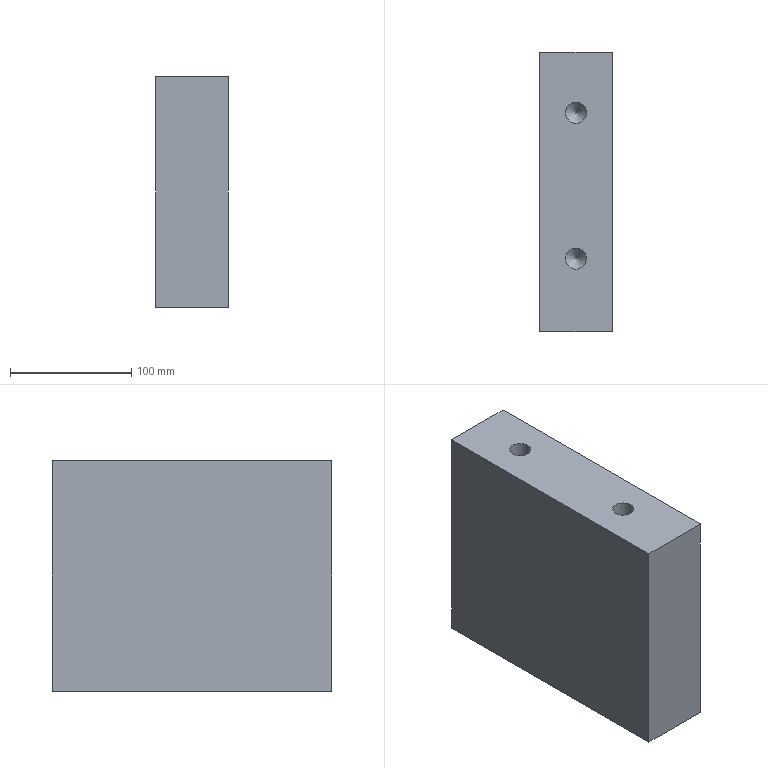Part | STEP file | lll_id4394_x_t | 1 solid | 12 faces | box 60 x 230 x 190 mm | volume 2590106 mm3 | plane 6 | cylinder 3 | cone 3 | commonest cylinder face diameters 17.506 x2 17.505 x1
STEP:
#1=CARTESIAN_POINT('',(517.435,370.,-370.));
#2=VERTEX_POINT('',#1);
#3=CARTESIAN_POINT('',(577.435,370.,-370.));
#4=VERTEX_POINT('',#3);
#5=CARTESIAN_POINT('',(2763.751,370.,-370.));
#6=DIRECTION('',(1.,0.,0.));
#7=VECTOR('',#6,1.);
#8=LINE('',#5,#7);
#9=EDGE_CURVE('',#2,#4,#8,.T.);
#10=ORIENTED_EDGE('',*,*,#9,.F.);
#11=CARTESIAN_POINT('',(517.435,600.,-370.));
#12=VERTEX_POINT('',#11);
#13=CARTESIAN_POINT('',(517.435,1.,-370.));
#14=DIRECTION('',(0.,-1.,0.));
#15=VECTOR('',#14,1.);
#16=LINE('',#13,#15);
#17=EDGE_CURVE('',#12,#2,#16,.T.);
#18=ORIENTED_EDGE('',*,*,#17,.F.);
#19=CARTESIAN_POINT('',(577.435,600.,-370.));
#20=VERTEX_POINT('',#19);
#21=CARTESIAN_POINT('',(-3392.565,600.,-370.));
#22=DIRECTION('',(1.,0.,0.));
#23=VECTOR('',#22,1.);
#24=LINE('',#21,#23);
#25=EDGE_CURVE('',#12,#20,#24,.T.);
#26=ORIENTED_EDGE('',*,*,#25,.T.);
#27=CARTESIAN_POINT('',(577.435,600.,-370.));
#28=DIRECTION('',(0.,-1.,0.));
#29=VECTOR('',#28,1.);
#30=LINE('',#27,#29);
#31=EDGE_CURVE('',#20,#4,#30,.T.);
#32=ORIENTED_EDGE('',*,*,#31,.T.);
#33=EDGE_LOOP('',(#10,#18,#26,#32));
#34=FACE_BOUND('',#33,.T.);
#35=CARTESIAN_POINT('',(556.188,550.,-370.));
#36=VERTEX_POINT('',#35);
#37=CARTESIAN_POINT('',(547.435,550.,-370.));
#38=DIRECTION('',(0.,0.,1.));
#39=DIRECTION('',(1.,0.,0.));
#40=AXIS2_PLACEMENT_3D('',#37,#38,#39);
#41=CIRCLE('',#40,8.752);
#42=EDGE_CURVE('',#36,#36,#41,.T.);
#43=ORIENTED_EDGE('',*,*,#42,.T.);
#44=EDGE_LOOP('',(#43));
#45=FACE_BOUND('',#44,.T.);
#46=CARTESIAN_POINT('',(2763.751,1.,-370.));
#47=DIRECTION('',(0.,0.,-1.));
#48=DIRECTION('',(-1.,0.,0.));
#49=AXIS2_PLACEMENT_3D('',#46,#47,#48);
#50=PLANE('',#49);
#51=ADVANCED_FACE('',(#34,#45),#50,.T.);
#52=CARTESIAN_POINT('',(517.435,600.,-180.));
#53=VERTEX_POINT('',#52);
#54=CARTESIAN_POINT('',(517.435,600.,-182.5));
#55=DIRECTION('',(0.,0.,1.));
#56=VECTOR('',#55,1.);
#57=LINE('',#54,#56);
#58=EDGE_CURVE('',#12,#53,#57,.T.);
#59=ORIENTED_EDGE('',*,*,#58,.T.);
#60=CARTESIAN_POINT('',(577.435,600.,-180.));
#61=VERTEX_POINT('',#60);
#62=CARTESIAN_POINT('',(2763.751,600.,-180.));
#63=DIRECTION('',(1.,0.,0.));
#64=VECTOR('',#63,1.);
#65=LINE('',#62,#64);
#66=EDGE_CURVE('',#53,#61,#65,.T.);
#67=ORIENTED_EDGE('',*,*,#66,.T.);
#68=CARTESIAN_POINT('',(577.435,600.,-182.5));
#69=DIRECTION('',(0.,0.,-1.));
#70=VECTOR('',#69,1.);
#71=LINE('',#68,#70);
#72=EDGE_CURVE('',#61,#20,#71,.T.);
#73=ORIENTED_EDGE('',*,*,#72,.T.);
#74=ORIENTED_EDGE('',*,*,#25,.F.);
#75=EDGE_LOOP('',(#59,#67,#73,#74));
#76=FACE_OUTER_BOUND('',#75,.T.);
#77=CARTESIAN_POINT('',(-3392.565,600.,-182.5));
#78=DIRECTION('',(0.,1.,0.));
#79=DIRECTION('',(0.,0.,1.));
#80=AXIS2_PLACEMENT_3D('',#77,#78,#79);
#81=PLANE('',#80);
#82=ADVANCED_FACE('',(#76),#81,.T.);
#83=CARTESIAN_POINT('',(538.682,430.,-180.));
#84=VERTEX_POINT('',#83);
#85=CARTESIAN_POINT('',(547.435,430.,-180.));
#86=DIRECTION('',(0.,0.,-1.));
#87=DIRECTION('',(-1.,0.,0.));
#88=AXIS2_PLACEMENT_3D('',#85,#86,#87);
#89=CIRCLE('',#88,8.753);
#90=EDGE_CURVE('',#84,#84,#89,.T.);
#91=ORIENTED_EDGE('',*,*,#90,.T.);
#92=EDGE_LOOP('',(#91));
#93=FACE_BOUND('',#92,.T.);
#94=CARTESIAN_POINT('',(538.682,550.,-180.));
#95=VERTEX_POINT('',#94);
#96=CARTESIAN_POINT('',(547.435,550.,-180.));
#97=DIRECTION('',(0.,0.,-1.));
#98=DIRECTION('',(-1.,0.,0.));
#99=AXIS2_PLACEMENT_3D('',#96,#97,#98);
#100=CIRCLE('',#99,8.753);
#101=EDGE_CURVE('',#95,#95,#100,.T.);
#102=ORIENTED_EDGE('',*,*,#101,.T.);
#103=EDGE_LOOP('',(#102));
#104=FACE_BOUND('',#103,.T.);
#105=CARTESIAN_POINT('',(517.435,370.,-180.));
#106=VERTEX_POINT('',#105);
#107=CARTESIAN_POINT('',(517.435,0.,-180.));
#108=DIRECTION('',(0.,1.,0.));
#109=VECTOR('',#108,1.);
#110=LINE('',#107,#109);
#111=EDGE_CURVE('',#106,#53,#110,.T.);
#112=ORIENTED_EDGE('',*,*,#111,.F.);
#113=CARTESIAN_POINT('',(577.435,370.,-180.));
#114=VERTEX_POINT('',#113);
#115=CARTESIAN_POINT('',(2763.751,370.,-180.));
#116=DIRECTION('',(1.,0.,0.));
#117=VECTOR('',#116,1.);
#118=LINE('',#115,#117);
#119=EDGE_CURVE('',#106,#114,#118,.T.);
#120=ORIENTED_EDGE('',*,*,#119,.T.);
#121=CARTESIAN_POINT('',(577.435,1.,-180.));
#122=DIRECTION('',(0.,-1.,0.));
#123=VECTOR('',#122,1.);
#124=LINE('',#121,#123);
#125=EDGE_CURVE('',#61,#114,#124,.T.);
#126=ORIENTED_EDGE('',*,*,#125,.F.);
#127=ORIENTED_EDGE('',*,*,#66,.F.);
#128=EDGE_LOOP('',(#112,#120,#126,#127));
#129=FACE_BOUND('',#128,.T.);
#130=CARTESIAN_POINT('',(2763.751,1.,-180.));
#131=DIRECTION('',(0.,0.,-1.));
#132=DIRECTION('',(-1.,0.,0.));
#133=AXIS2_PLACEMENT_3D('',#130,#131,#132);
#134=PLANE('',#133);
#135=ADVANCED_FACE('',(#93,#104,#129),#134,.F.);
#136=CARTESIAN_POINT('',(577.435,370.,-182.5));
#137=DIRECTION('',(0.,0.,-1.));
#138=VECTOR('',#137,1.);
#139=LINE('',#136,#138);
#140=EDGE_CURVE('',#114,#4,#139,.T.);
#141=ORIENTED_EDGE('',*,*,#140,.T.);
#142=ORIENTED_EDGE('',*,*,#31,.F.);
#143=ORIENTED_EDGE('',*,*,#72,.F.);
#144=ORIENTED_EDGE('',*,*,#125,.T.);
#145=EDGE_LOOP('',(#141,#142,#143,#144));
#146=FACE_OUTER_BOUND('',#145,.T.);
#147=CARTESIAN_POINT('',(577.435,600.,-182.5));
#148=DIRECTION('',(1.,0.,0.));
#149=DIRECTION('',(0.,0.,-1.));
#150=AXIS2_PLACEMENT_3D('',#147,#148,#149);
#151=PLANE('',#150);
#152=ADVANCED_FACE('',(#146),#151,.T.);
#153=ORIENTED_EDGE('',*,*,#17,.T.);
#154=CARTESIAN_POINT('',(517.435,370.,-251.25));
#155=DIRECTION('',(0.,0.,1.));
#156=VECTOR('',#155,1.);
#157=LINE('',#154,#156);
#158=EDGE_CURVE('',#2,#106,#157,.T.);
#159=ORIENTED_EDGE('',*,*,#158,.T.);
#160=ORIENTED_EDGE('',*,*,#111,.T.);
#161=ORIENTED_EDGE('',*,*,#58,.F.);
#162=EDGE_LOOP('',(#153,#159,#160,#161));
#163=FACE_OUTER_BOUND('',#162,.T.);
#164=CARTESIAN_POINT('',(517.435,0.,-251.25));
#165=DIRECTION('',(1.,0.,0.));
#166=DIRECTION('',(0.,0.,-1.));
#167=AXIS2_PLACEMENT_3D('',#164,#165,#166);
#168=PLANE('',#167);
#169=ADVANCED_FACE('',(#163),#168,.F.);
#170=ORIENTED_EDGE('',*,*,#158,.F.);
#171=ORIENTED_EDGE('',*,*,#9,.T.);
#172=ORIENTED_EDGE('',*,*,#140,.F.);
#173=ORIENTED_EDGE('',*,*,#119,.F.);
#174=EDGE_LOOP('',(#170,#171,#172,#173));
#175=FACE_OUTER_BOUND('',#174,.T.);
#176=CARTESIAN_POINT('',(547.435,370.,-250.));
#177=DIRECTION('',(0.,1.,0.));
#178=DIRECTION('',(0.,0.,1.));
#179=AXIS2_PLACEMENT_3D('',#176,#177,#178);
#180=PLANE('',#179);
#181=ADVANCED_FACE('',(#175),#180,.F.);
#182=CARTESIAN_POINT('',(556.188,550.,-328.747));
#183=VERTEX_POINT('',#182);
#184=CARTESIAN_POINT('',(547.435,550.,-328.747));
#185=DIRECTION('',(0.,0.,1.));
#186=DIRECTION('',(1.,0.,0.));
#187=AXIS2_PLACEMENT_3D('',#184,#185,#186);
#188=CIRCLE('',#187,8.752);
#189=EDGE_CURVE('',#183,#183,#188,.T.);
#190=ORIENTED_EDGE('',*,*,#189,.T.);
#191=EDGE_LOOP('',(#190));
#192=FACE_BOUND('',#191,.T.);
#193=ORIENTED_EDGE('',*,*,#42,.F.);
#194=EDGE_LOOP('',(#193));
#195=FACE_BOUND('',#194,.T.);
#196=CARTESIAN_POINT('',(547.435,550.,-370.));
#197=DIRECTION('',(0.,0.,1.));
#198=DIRECTION('',(-1.,0.,0.));
#199=AXIS2_PLACEMENT_3D('',#196,#197,#198);
#200=CYLINDRICAL_SURFACE('',#199,8.752);
#201=ADVANCED_FACE('',(#192,#195),#200,.F.);
#202=CARTESIAN_POINT('',(547.435,550.,-319.994));
#203=VERTEX_POINT('',#202);
#204=VERTEX_LOOP('',#203);
#205=FACE_BOUND('',#204,.T.);
#206=ORIENTED_EDGE('',*,*,#189,.F.);
#207=EDGE_LOOP('',(#206));
#208=FACE_BOUND('',#207,.T.);
#209=CARTESIAN_POINT('',(547.435,550.,-328.747));
#210=DIRECTION('',(0.,0.,-1.));
#211=DIRECTION('',(1.,0.,0.));
#212=AXIS2_PLACEMENT_3D('',#209,#210,#211);
#213=CONICAL_SURFACE('',#212,8.752,45.);
#214=ADVANCED_FACE('',(#205,#208),#213,.F.);
#215=CARTESIAN_POINT('',(538.682,550.,-221.253));
#216=VERTEX_POINT('',#215);
#217=CARTESIAN_POINT('',(547.435,550.,-221.253));
#218=DIRECTION('',(0.,0.,-1.));
#219=DIRECTION('',(-1.,0.,0.));
#220=AXIS2_PLACEMENT_3D('',#217,#218,#219);
#221=CIRCLE('',#220,8.753);
#222=EDGE_CURVE('',#216,#216,#221,.T.);
#223=ORIENTED_EDGE('',*,*,#222,.T.);
#224=EDGE_LOOP('',(#223));
#225=FACE_BOUND('',#224,.T.);
#226=ORIENTED_EDGE('',*,*,#101,.F.);
#227=EDGE_LOOP('',(#226));
#228=FACE_BOUND('',#227,.T.);
#229=CARTESIAN_POINT('',(547.435,550.,-180.));
#230=DIRECTION('',(0.,0.,-1.));
#231=DIRECTION('',(1.,0.,0.));
#232=AXIS2_PLACEMENT_3D('',#229,#230,#231);
#233=CYLINDRICAL_SURFACE('',#232,8.753);
#234=ADVANCED_FACE('',(#225,#228),#233,.F.);
#235=CARTESIAN_POINT('',(547.435,550.,-230.006));
#236=VERTEX_POINT('',#235);
#237=VERTEX_LOOP('',#236);
#238=FACE_BOUND('',#237,.T.);
#239=ORIENTED_EDGE('',*,*,#222,.F.);
#240=EDGE_LOOP('',(#239));
#241=FACE_BOUND('',#240,.T.);
#242=CARTESIAN_POINT('',(547.435,550.,-221.253));
#243=DIRECTION('',(0.,0.,1.));
#244=DIRECTION('',(-1.,0.,0.));
#245=AXIS2_PLACEMENT_3D('',#242,#243,#244);
#246=CONICAL_SURFACE('',#245,8.753,45.);
#247=ADVANCED_FACE('',(#238,#241),#246,.F.);
#248=CARTESIAN_POINT('',(538.682,430.,-221.253));
#249=VERTEX_POINT('',#248);
#250=CARTESIAN_POINT('',(547.435,430.,-221.253));
#251=DIRECTION('',(0.,0.,-1.));
#252=DIRECTION('',(-1.,0.,0.));
#253=AXIS2_PLACEMENT_3D('',#250,#251,#252);
#254=CIRCLE('',#253,8.753);
#255=EDGE_CURVE('',#249,#249,#254,.T.);
#256=ORIENTED_EDGE('',*,*,#255,.T.);
#257=EDGE_LOOP('',(#256));
#258=FACE_BOUND('',#257,.T.);
#259=ORIENTED_EDGE('',*,*,#90,.F.);
#260=EDGE_LOOP('',(#259));
#261=FACE_BOUND('',#260,.T.);
#262=CARTESIAN_POINT('',(547.435,430.,-180.));
#263=DIRECTION('',(0.,0.,-1.));
#264=DIRECTION('',(1.,0.,0.));
#265=AXIS2_PLACEMENT_3D('',#262,#263,#264);
#266=CYLINDRICAL_SURFACE('',#265,8.753);
#267=ADVANCED_FACE('',(#258,#261),#266,.F.);
#268=CARTESIAN_POINT('',(547.435,430.,-230.006));
#269=VERTEX_POINT('',#268);
#270=VERTEX_LOOP('',#269);
#271=FACE_BOUND('',#270,.T.);
#272=ORIENTED_EDGE('',*,*,#255,.F.);
#273=EDGE_LOOP('',(#272));
#274=FACE_BOUND('',#273,.T.);
#275=CARTESIAN_POINT('',(547.435,430.,-221.253));
#276=DIRECTION('',(0.,0.,1.));
#277=DIRECTION('',(-1.,0.,0.));
#278=AXIS2_PLACEMENT_3D('',#275,#276,#277);
#279=CONICAL_SURFACE('',#278,8.753,45.);
#280=ADVANCED_FACE('',(#271,#274),#279,.F.);
#281=CLOSED_SHELL('',(#51,#82,#135,#152,#169,#181,#201,#214,#234,#247,#267,#280));
#282=MANIFOLD_SOLID_BREP('',#281);
#283=(LENGTH_UNIT()NAMED_UNIT(*)SI_UNIT(.MILLI.,.METRE.));
#284=UNCERTAINTY_MEASURE_WITH_UNIT(LENGTH_MEASURE(0.00002),#283,'','');
#285=(NAMED_UNIT(*)PLANE_ANGLE_UNIT()SI_UNIT($,.RADIAN.));
#286=PLANE_ANGLE_MEASURE_WITH_UNIT(PLANE_ANGLE_MEASURE(0.01745),#285);
#287=DIMENSIONAL_EXPONENTS(0.,0.,0.,0.,0.,0.,0.);
#288=(CONVERSION_BASED_UNIT('DEGREE',#286)NAMED_UNIT(#287)PLANE_ANGLE_UNIT());
#289=(NAMED_UNIT(*)SI_UNIT($,.STERADIAN.)SOLID_ANGLE_UNIT());
#290=(GEOMETRIC_REPRESENTATION_CONTEXT(3)GLOBAL_UNCERTAINTY_ASSIGNED_CONTEXT((#284))GLOBAL_UNIT_ASSIGNED_CONTEXT((#283,#288,#289))REPRESENTATION_CONTEXT('',''));
#291=ADVANCED_BREP_SHAPE_REPRESENTATION('',(#282),#290);